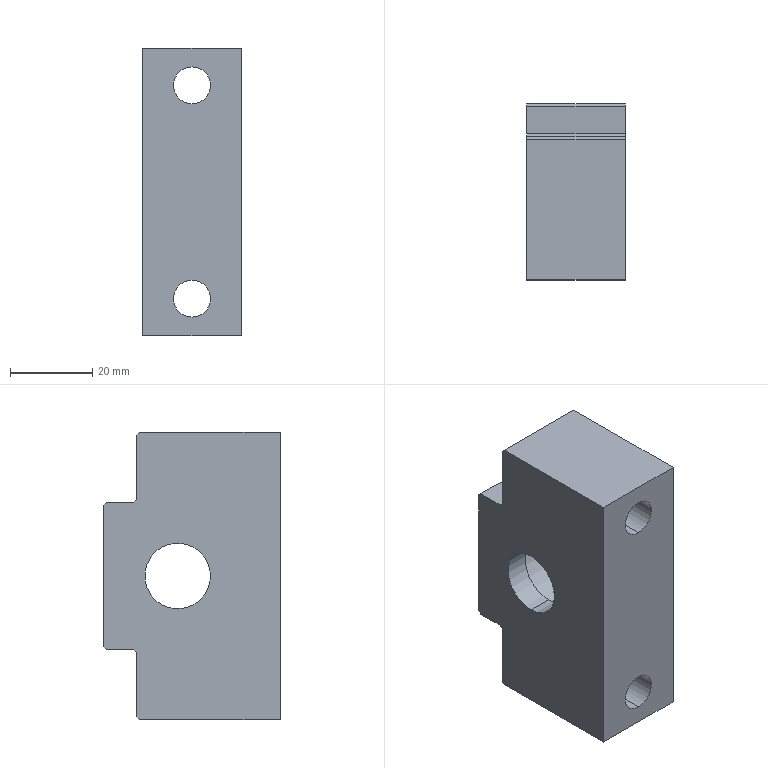Part | STEP file | BSW12bsw | 1 solid | 31 faces | box 24 x 43 x 70 mm | volume 48051 mm3 | plane 19 | cylinder 12 | commonest cylinder face diameters 9 x4 14 x4 16 x2 26.6 x2
STEP:
#1=CARTESIAN_POINT('',(12.,-25.,21.5));
#2=VERTEX_POINT('',#1);
#3=CARTESIAN_POINT('',(12.,-25.,30.5));
#4=VERTEX_POINT('',#3);
#5=CARTESIAN_POINT('',(12.,-25.,26.));
#6=DIRECTION('',(0.,1.,0.));
#7=DIRECTION('',(0.,0.,1.));
#8=AXIS2_PLACEMENT_3D('',#5,#6,#7);
#9=CIRCLE('',#8,4.5);
#10=EDGE_CURVE('',#2,#4,#9,.T.);
#11=ORIENTED_EDGE('',*,*,#10,.F.);
#12=CARTESIAN_POINT('',(12.,-1.,21.5));
#13=VERTEX_POINT('',#12);
#14=CARTESIAN_POINT('',(12.,-25.,21.5));
#15=DIRECTION('',(0.,1.,0.));
#16=VECTOR('',#15,1000.);
#17=LINE('',#14,#16);
#18=EDGE_CURVE('',#2,#13,#17,.T.);
#19=ORIENTED_EDGE('',*,*,#18,.T.);
#20=CARTESIAN_POINT('',(12.,-1.,30.5));
#21=VERTEX_POINT('',#20);
#22=CARTESIAN_POINT('',(12.,-1.,26.));
#23=DIRECTION('',(0.,1.,0.));
#24=DIRECTION('',(0.,0.,1.));
#25=AXIS2_PLACEMENT_3D('',#22,#23,#24);
#26=CIRCLE('',#25,4.5);
#27=EDGE_CURVE('',#13,#21,#26,.T.);
#28=ORIENTED_EDGE('',*,*,#27,.T.);
#29=CARTESIAN_POINT('',(12.,-25.,30.5));
#30=DIRECTION('',(0.,1.,0.));
#31=VECTOR('',#30,1000.);
#32=LINE('',#29,#31);
#33=EDGE_CURVE('',#4,#21,#32,.T.);
#34=ORIENTED_EDGE('',*,*,#33,.F.);
#35=EDGE_LOOP('',(#11,#19,#28,#34));
#36=FACE_OUTER_BOUND('',#35,.T.);
#37=CARTESIAN_POINT('',(12.,-25.,26.));
#38=DIRECTION('',(0.,1.,0.));
#39=DIRECTION('',(0.,0.,1.));
#40=AXIS2_PLACEMENT_3D('',#37,#38,#39);
#41=CYLINDRICAL_SURFACE('',#40,4.5);
#42=ADVANCED_FACE('',(#36),#41,.F.);
#43=CARTESIAN_POINT('',(12.,-1.,19.));
#44=VERTEX_POINT('',#43);
#45=CARTESIAN_POINT('',(12.,-1.,33.));
#46=VERTEX_POINT('',#45);
#47=CARTESIAN_POINT('',(12.,-1.,26.));
#48=DIRECTION('',(0.,1.,0.));
#49=DIRECTION('',(0.,0.,1.));
#50=AXIS2_PLACEMENT_3D('',#47,#48,#49);
#51=CIRCLE('',#50,7.);
#52=EDGE_CURVE('',#44,#46,#51,.T.);
#53=ORIENTED_EDGE('',*,*,#52,.F.);
#54=CARTESIAN_POINT('',(12.,10.,19.));
#55=VERTEX_POINT('',#54);
#56=CARTESIAN_POINT('',(12.,-25.,19.));
#57=DIRECTION('',(0.,1.,0.));
#58=VECTOR('',#57,1000.);
#59=LINE('',#56,#58);
#60=EDGE_CURVE('',#44,#55,#59,.T.);
#61=ORIENTED_EDGE('',*,*,#60,.T.);
#62=CARTESIAN_POINT('',(12.,10.,33.));
#63=VERTEX_POINT('',#62);
#64=CARTESIAN_POINT('',(12.,10.,26.));
#65=DIRECTION('',(0.,1.,0.));
#66=DIRECTION('',(0.,0.,1.));
#67=AXIS2_PLACEMENT_3D('',#64,#65,#66);
#68=CIRCLE('',#67,7.);
#69=EDGE_CURVE('',#55,#63,#68,.T.);
#70=ORIENTED_EDGE('',*,*,#69,.T.);
#71=CARTESIAN_POINT('',(12.,-25.,33.));
#72=DIRECTION('',(0.,1.,0.));
#73=VECTOR('',#72,1000.);
#74=LINE('',#71,#73);
#75=EDGE_CURVE('',#46,#63,#74,.T.);
#76=ORIENTED_EDGE('',*,*,#75,.F.);
#77=EDGE_LOOP('',(#53,#61,#70,#76));
#78=FACE_OUTER_BOUND('',#77,.T.);
#79=CARTESIAN_POINT('',(12.,-25.,26.));
#80=DIRECTION('',(0.,1.,0.));
#81=DIRECTION('',(0.,0.,1.));
#82=AXIS2_PLACEMENT_3D('',#79,#80,#81);
#83=CYLINDRICAL_SURFACE('',#82,7.);
#84=ADVANCED_FACE('',(#78),#83,.F.);
#85=CARTESIAN_POINT('',(12.,-25.,-30.5));
#86=VERTEX_POINT('',#85);
#87=CARTESIAN_POINT('',(12.,-25.,-21.5));
#88=VERTEX_POINT('',#87);
#89=CARTESIAN_POINT('',(12.,-25.,-26.));
#90=DIRECTION('',(0.,1.,0.));
#91=DIRECTION('',(0.,0.,1.));
#92=AXIS2_PLACEMENT_3D('',#89,#90,#91);
#93=CIRCLE('',#92,4.5);
#94=EDGE_CURVE('',#86,#88,#93,.T.);
#95=ORIENTED_EDGE('',*,*,#94,.F.);
#96=CARTESIAN_POINT('',(12.,-1.,-30.5));
#97=VERTEX_POINT('',#96);
#98=CARTESIAN_POINT('',(12.,-25.,-30.5));
#99=DIRECTION('',(0.,1.,0.));
#100=VECTOR('',#99,1000.);
#101=LINE('',#98,#100);
#102=EDGE_CURVE('',#86,#97,#101,.T.);
#103=ORIENTED_EDGE('',*,*,#102,.T.);
#104=CARTESIAN_POINT('',(12.,-1.,-21.5));
#105=VERTEX_POINT('',#104);
#106=CARTESIAN_POINT('',(12.,-1.,-26.));
#107=DIRECTION('',(0.,1.,0.));
#108=DIRECTION('',(0.,0.,1.));
#109=AXIS2_PLACEMENT_3D('',#106,#107,#108);
#110=CIRCLE('',#109,4.5);
#111=EDGE_CURVE('',#97,#105,#110,.T.);
#112=ORIENTED_EDGE('',*,*,#111,.T.);
#113=CARTESIAN_POINT('',(12.,-25.,-21.5));
#114=DIRECTION('',(0.,1.,0.));
#115=VECTOR('',#114,1000.);
#116=LINE('',#113,#115);
#117=EDGE_CURVE('',#88,#105,#116,.T.);
#118=ORIENTED_EDGE('',*,*,#117,.F.);
#119=EDGE_LOOP('',(#95,#103,#112,#118));
#120=FACE_OUTER_BOUND('',#119,.T.);
#121=CARTESIAN_POINT('',(12.,-25.,-26.));
#122=DIRECTION('',(0.,1.,0.));
#123=DIRECTION('',(0.,0.,1.));
#124=AXIS2_PLACEMENT_3D('',#121,#122,#123);
#125=CYLINDRICAL_SURFACE('',#124,4.5);
#126=ADVANCED_FACE('',(#120),#125,.F.);
#127=CARTESIAN_POINT('',(12.,-1.,-33.));
#128=VERTEX_POINT('',#127);
#129=CARTESIAN_POINT('',(12.,-1.,-19.));
#130=VERTEX_POINT('',#129);
#131=CARTESIAN_POINT('',(12.,-1.,-26.));
#132=DIRECTION('',(0.,1.,0.));
#133=DIRECTION('',(0.,0.,1.));
#134=AXIS2_PLACEMENT_3D('',#131,#132,#133);
#135=CIRCLE('',#134,7.);
#136=EDGE_CURVE('',#128,#130,#135,.T.);
#137=ORIENTED_EDGE('',*,*,#136,.F.);
#138=CARTESIAN_POINT('',(12.,10.,-33.));
#139=VERTEX_POINT('',#138);
#140=CARTESIAN_POINT('',(12.,-25.,-33.));
#141=DIRECTION('',(0.,1.,0.));
#142=VECTOR('',#141,1000.);
#143=LINE('',#140,#142);
#144=EDGE_CURVE('',#128,#139,#143,.T.);
#145=ORIENTED_EDGE('',*,*,#144,.T.);
#146=CARTESIAN_POINT('',(12.,10.,-19.));
#147=VERTEX_POINT('',#146);
#148=CARTESIAN_POINT('',(12.,10.,-26.));
#149=DIRECTION('',(0.,1.,0.));
#150=DIRECTION('',(0.,0.,1.));
#151=AXIS2_PLACEMENT_3D('',#148,#149,#150);
#152=CIRCLE('',#151,7.);
#153=EDGE_CURVE('',#139,#147,#152,.T.);
#154=ORIENTED_EDGE('',*,*,#153,.T.);
#155=CARTESIAN_POINT('',(12.,-25.,-19.));
#156=DIRECTION('',(0.,1.,0.));
#157=VECTOR('',#156,1000.);
#158=LINE('',#155,#157);
#159=EDGE_CURVE('',#130,#147,#158,.T.);
#160=ORIENTED_EDGE('',*,*,#159,.F.);
#161=EDGE_LOOP('',(#137,#145,#154,#160));
#162=FACE_OUTER_BOUND('',#161,.T.);
#163=CARTESIAN_POINT('',(12.,-25.,-26.));
#164=DIRECTION('',(0.,1.,0.));
#165=DIRECTION('',(0.,0.,1.));
#166=AXIS2_PLACEMENT_3D('',#163,#164,#165);
#167=CYLINDRICAL_SURFACE('',#166,7.);
#168=ADVANCED_FACE('',(#162),#167,.F.);
#169=CARTESIAN_POINT('',(24.,0.,-13.3));
#170=VERTEX_POINT('',#169);
#171=CARTESIAN_POINT('',(24.,0.,13.3));
#172=VERTEX_POINT('',#171);
#173=CARTESIAN_POINT('',(24.,0.,0.));
#174=DIRECTION('',(-1.,0.,0.));
#175=DIRECTION('',(0.,0.,1.));
#176=AXIS2_PLACEMENT_3D('',#173,#174,#175);
#177=CIRCLE('',#176,13.3);
#178=EDGE_CURVE('',#170,#172,#177,.T.);
#179=ORIENTED_EDGE('',*,*,#178,.F.);
#180=CARTESIAN_POINT('',(6.,0.,-13.3));
#181=VERTEX_POINT('',#180);
#182=CARTESIAN_POINT('',(24.,0.,-13.3));
#183=DIRECTION('',(-1.,0.,0.));
#184=VECTOR('',#183,1000.);
#185=LINE('',#182,#184);
#186=EDGE_CURVE('',#170,#181,#185,.T.);
#187=ORIENTED_EDGE('',*,*,#186,.T.);
#188=CARTESIAN_POINT('',(6.,0.,13.3));
#189=VERTEX_POINT('',#188);
#190=CARTESIAN_POINT('',(6.,0.,0.));
#191=DIRECTION('',(-1.,0.,0.));
#192=DIRECTION('',(0.,0.,1.));
#193=AXIS2_PLACEMENT_3D('',#190,#191,#192);
#194=CIRCLE('',#193,13.3);
#195=EDGE_CURVE('',#181,#189,#194,.T.);
#196=ORIENTED_EDGE('',*,*,#195,.T.);
#197=CARTESIAN_POINT('',(24.,0.,13.3));
#198=DIRECTION('',(-1.,0.,0.));
#199=VECTOR('',#198,1000.);
#200=LINE('',#197,#199);
#201=EDGE_CURVE('',#172,#189,#200,.T.);
#202=ORIENTED_EDGE('',*,*,#201,.F.);
#203=EDGE_LOOP('',(#179,#187,#196,#202));
#204=FACE_OUTER_BOUND('',#203,.T.);
#205=CARTESIAN_POINT('',(24.,0.,0.));
#206=DIRECTION('',(-1.,0.,0.));
#207=DIRECTION('',(0.,0.,1.));
#208=AXIS2_PLACEMENT_3D('',#205,#206,#207);
#209=CYLINDRICAL_SURFACE('',#208,13.3);
#210=ADVANCED_FACE('',(#204),#209,.F.);
#211=CARTESIAN_POINT('',(6.,0.,-8.));
#212=VERTEX_POINT('',#211);
#213=CARTESIAN_POINT('',(6.,0.,8.));
#214=VERTEX_POINT('',#213);
#215=CARTESIAN_POINT('',(6.,0.,0.));
#216=DIRECTION('',(-1.,0.,0.));
#217=DIRECTION('',(0.,0.,1.));
#218=AXIS2_PLACEMENT_3D('',#215,#216,#217);
#219=CIRCLE('',#218,8.);
#220=EDGE_CURVE('',#212,#214,#219,.T.);
#221=ORIENTED_EDGE('',*,*,#220,.F.);
#222=CARTESIAN_POINT('',(0.,0.,-8.));
#223=VERTEX_POINT('',#222);
#224=CARTESIAN_POINT('',(24.,0.,-8.));
#225=DIRECTION('',(-1.,0.,0.));
#226=VECTOR('',#225,1000.);
#227=LINE('',#224,#226);
#228=EDGE_CURVE('',#212,#223,#227,.T.);
#229=ORIENTED_EDGE('',*,*,#228,.T.);
#230=CARTESIAN_POINT('',(0.,0.,8.));
#231=VERTEX_POINT('',#230);
#232=CARTESIAN_POINT('',(0.,0.,0.));
#233=DIRECTION('',(-1.,0.,0.));
#234=DIRECTION('',(0.,0.,1.));
#235=AXIS2_PLACEMENT_3D('',#232,#233,#234);
#236=CIRCLE('',#235,8.);
#237=EDGE_CURVE('',#223,#231,#236,.T.);
#238=ORIENTED_EDGE('',*,*,#237,.T.);
#239=CARTESIAN_POINT('',(24.,0.,8.));
#240=DIRECTION('',(-1.,0.,0.));
#241=VECTOR('',#240,1000.);
#242=LINE('',#239,#241);
#243=EDGE_CURVE('',#214,#231,#242,.T.);
#244=ORIENTED_EDGE('',*,*,#243,.F.);
#245=EDGE_LOOP('',(#221,#229,#238,#244));
#246=FACE_OUTER_BOUND('',#245,.T.);
#247=CARTESIAN_POINT('',(24.,0.,0.));
#248=DIRECTION('',(-1.,0.,0.));
#249=DIRECTION('',(0.,0.,1.));
#250=AXIS2_PLACEMENT_3D('',#247,#248,#249);
#251=CYLINDRICAL_SURFACE('',#250,8.);
#252=ADVANCED_FACE('',(#246),#251,.F.);
#253=CARTESIAN_POINT('',(12.,-25.,-26.));
#254=DIRECTION('',(0.,1.,0.));
#255=DIRECTION('',(0.,0.,1.));
#256=AXIS2_PLACEMENT_3D('',#253,#254,#255);
#257=CIRCLE('',#256,4.5);
#258=EDGE_CURVE('',#88,#86,#257,.T.);
#259=ORIENTED_EDGE('',*,*,#258,.T.);
#260=ORIENTED_EDGE('',*,*,#94,.T.);
#261=EDGE_LOOP('',(#259,#260));
#262=FACE_BOUND('',#261,.T.);
#263=CARTESIAN_POINT('',(0.,-25.,35.));
#264=VERTEX_POINT('',#263);
#265=CARTESIAN_POINT('',(0.,-25.,-35.));
#266=VERTEX_POINT('',#265);
#267=CARTESIAN_POINT('',(0.,-25.,35.));
#268=DIRECTION('',(0.,0.,-1.));
#269=VECTOR('',#268,1000.);
#270=LINE('',#267,#269);
#271=EDGE_CURVE('',#264,#266,#270,.T.);
#272=ORIENTED_EDGE('',*,*,#271,.T.);
#273=CARTESIAN_POINT('',(24.,-25.,-35.));
#274=VERTEX_POINT('',#273);
#275=CARTESIAN_POINT('',(24.,-25.,-35.));
#276=DIRECTION('',(-1.,0.,0.));
#277=VECTOR('',#276,1000.);
#278=LINE('',#275,#277);
#279=EDGE_CURVE('',#274,#266,#278,.T.);
#280=ORIENTED_EDGE('',*,*,#279,.F.);
#281=CARTESIAN_POINT('',(24.,-25.,35.));
#282=VERTEX_POINT('',#281);
#283=CARTESIAN_POINT('',(24.,-25.,35.));
#284=DIRECTION('',(0.,0.,-1.));
#285=VECTOR('',#284,1000.);
#286=LINE('',#283,#285);
#287=EDGE_CURVE('',#282,#274,#286,.T.);
#288=ORIENTED_EDGE('',*,*,#287,.F.);
#289=CARTESIAN_POINT('',(24.,-25.,35.));
#290=DIRECTION('',(-1.,0.,0.));
#291=VECTOR('',#290,1000.);
#292=LINE('',#289,#291);
#293=EDGE_CURVE('',#282,#264,#292,.T.);
#294=ORIENTED_EDGE('',*,*,#293,.T.);
#295=EDGE_LOOP('',(#272,#280,#288,#294));
#296=FACE_OUTER_BOUND('',#295,.T.);
#297=CARTESIAN_POINT('',(12.,-25.,26.));
#298=DIRECTION('',(0.,1.,0.));
#299=DIRECTION('',(0.,0.,1.));
#300=AXIS2_PLACEMENT_3D('',#297,#298,#299);
#301=CIRCLE('',#300,4.5);
#302=EDGE_CURVE('',#4,#2,#301,.T.);
#303=ORIENTED_EDGE('',*,*,#302,.T.);
#304=ORIENTED_EDGE('',*,*,#10,.T.);
#305=EDGE_LOOP('',(#303,#304));
#306=FACE_BOUND('',#305,.T.);
#307=CARTESIAN_POINT('',(24.,-25.,35.));
#308=DIRECTION('',(0.,1.,0.));
#309=DIRECTION('',(0.,0.,1.));
#310=AXIS2_PLACEMENT_3D('',#307,#308,#309);
#311=PLANE('',#310);
#312=ADVANCED_FACE('',(#262,#296,#306),#311,.F.);
#313=CARTESIAN_POINT('',(0.,10.,18.7));
#314=VERTEX_POINT('',#313);
#315=CARTESIAN_POINT('',(0.,10.,34.3));
#316=VERTEX_POINT('',#315);
#317=CARTESIAN_POINT('',(0.,10.,18.7));
#318=DIRECTION('',(0.,0.,1.));
#319=VECTOR('',#318,1000.);
#320=LINE('',#317,#319);
#321=EDGE_CURVE('',#314,#316,#320,.T.);
#322=ORIENTED_EDGE('',*,*,#321,.T.);
#323=CARTESIAN_POINT('',(24.,10.,34.3));
#324=VERTEX_POINT('',#323);
#325=CARTESIAN_POINT('',(24.,10.,34.3));
#326=DIRECTION('',(-1.,0.,0.));
#327=VECTOR('',#326,1000.);
#328=LINE('',#325,#327);
#329=EDGE_CURVE('',#324,#316,#328,.T.);
#330=ORIENTED_EDGE('',*,*,#329,.F.);
#331=CARTESIAN_POINT('',(24.,10.,18.7));
#332=VERTEX_POINT('',#331);
#333=CARTESIAN_POINT('',(24.,10.,18.7));
#334=DIRECTION('',(0.,0.,1.));
#335=VECTOR('',#334,1000.);
#336=LINE('',#333,#335);
#337=EDGE_CURVE('',#332,#324,#336,.T.);
#338=ORIENTED_EDGE('',*,*,#337,.F.);
#339=CARTESIAN_POINT('',(24.,10.,18.7));
#340=DIRECTION('',(-1.,0.,0.));
#341=VECTOR('',#340,1000.);
#342=LINE('',#339,#341);
#343=EDGE_CURVE('',#332,#314,#342,.T.);
#344=ORIENTED_EDGE('',*,*,#343,.T.);
#345=EDGE_LOOP('',(#322,#330,#338,#344));
#346=FACE_OUTER_BOUND('',#345,.T.);
#347=CARTESIAN_POINT('',(12.,10.,26.));
#348=DIRECTION('',(0.,1.,0.));
#349=DIRECTION('',(0.,0.,1.));
#350=AXIS2_PLACEMENT_3D('',#347,#348,#349);
#351=CIRCLE('',#350,7.);
#352=EDGE_CURVE('',#63,#55,#351,.T.);
#353=ORIENTED_EDGE('',*,*,#352,.F.);
#354=ORIENTED_EDGE('',*,*,#69,.F.);
#355=EDGE_LOOP('',(#353,#354));
#356=FACE_BOUND('',#355,.T.);
#357=CARTESIAN_POINT('',(24.,10.,18.7));
#358=DIRECTION('',(0.,-1.,0.));
#359=DIRECTION('',(0.,0.,-1.));
#360=AXIS2_PLACEMENT_3D('',#357,#358,#359);
#361=PLANE('',#360);
#362=ADVANCED_FACE('',(#346,#356),#361,.F.);
#363=CARTESIAN_POINT('',(0.,10.,-34.3));
#364=VERTEX_POINT('',#363);
#365=CARTESIAN_POINT('',(0.,10.,-18.7));
#366=VERTEX_POINT('',#365);
#367=CARTESIAN_POINT('',(0.,10.,-34.3));
#368=DIRECTION('',(0.,0.,1.));
#369=VECTOR('',#368,1000.);
#370=LINE('',#367,#369);
#371=EDGE_CURVE('',#364,#366,#370,.T.);
#372=ORIENTED_EDGE('',*,*,#371,.T.);
#373=CARTESIAN_POINT('',(24.,10.,-18.7));
#374=VERTEX_POINT('',#373);
#375=CARTESIAN_POINT('',(24.,10.,-18.7));
#376=DIRECTION('',(-1.,0.,0.));
#377=VECTOR('',#376,1000.);
#378=LINE('',#375,#377);
#379=EDGE_CURVE('',#374,#366,#378,.T.);
#380=ORIENTED_EDGE('',*,*,#379,.F.);
#381=CARTESIAN_POINT('',(24.,10.,-34.3));
#382=VERTEX_POINT('',#381);
#383=CARTESIAN_POINT('',(24.,10.,-34.3));
#384=DIRECTION('',(0.,0.,1.));
#385=VECTOR('',#384,1000.);
#386=LINE('',#383,#385);
#387=EDGE_CURVE('',#382,#374,#386,.T.);
#388=ORIENTED_EDGE('',*,*,#387,.F.);
#389=CARTESIAN_POINT('',(24.,10.,-34.3));
#390=DIRECTION('',(-1.,0.,0.));
#391=VECTOR('',#390,1000.);
#392=LINE('',#389,#391);
#393=EDGE_CURVE('',#382,#364,#392,.T.);
#394=ORIENTED_EDGE('',*,*,#393,.T.);
#395=EDGE_LOOP('',(#372,#380,#388,#394));
#396=FACE_OUTER_BOUND('',#395,.T.);
#397=CARTESIAN_POINT('',(12.,10.,-26.));
#398=DIRECTION('',(0.,1.,0.));
#399=DIRECTION('',(0.,0.,1.));
#400=AXIS2_PLACEMENT_3D('',#397,#398,#399);
#401=CIRCLE('',#400,7.);
#402=EDGE_CURVE('',#147,#139,#401,.T.);
#403=ORIENTED_EDGE('',*,*,#402,.F.);
#404=ORIENTED_EDGE('',*,*,#153,.F.);
#405=EDGE_LOOP('',(#403,#404));
#406=FACE_BOUND('',#405,.T.);
#407=CARTESIAN_POINT('',(24.,10.,-34.3));
#408=DIRECTION('',(0.,-1.,0.));
#409=DIRECTION('',(0.,0.,-1.));
#410=AXIS2_PLACEMENT_3D('',#407,#408,#409);
#411=PLANE('',#410);
#412=ADVANCED_FACE('',(#396,#406),#411,.F.);
#413=CARTESIAN_POINT('',(24.,9.3,35.));
#414=VERTEX_POINT('',#413);
#415=CARTESIAN_POINT('',(24.,9.3,35.));
#416=DIRECTION('',(0.,-1.,0.));
#417=VECTOR('',#416,1000.);
#418=LINE('',#415,#417);
#419=EDGE_CURVE('',#414,#282,#418,.T.);
#420=ORIENTED_EDGE('',*,*,#419,.T.);
#421=ORIENTED_EDGE('',*,*,#287,.T.);
#422=CARTESIAN_POINT('',(24.,9.3,-35.));
#423=VERTEX_POINT('',#422);
#424=CARTESIAN_POINT('',(24.,-25.,-35.));
#425=DIRECTION('',(0.,1.,0.));
#426=VECTOR('',#425,1000.);
#427=LINE('',#424,#426);
#428=EDGE_CURVE('',#274,#423,#427,.T.);
#429=ORIENTED_EDGE('',*,*,#428,.T.);
#430=CARTESIAN_POINT('',(24.,9.3,-35.));
#431=DIRECTION('',(0.,0.7071,0.7071));
#432=VECTOR('',#431,1000.);
#433=LINE('',#430,#432);
#434=EDGE_CURVE('',#423,#382,#433,.T.);
#435=ORIENTED_EDGE('',*,*,#434,.T.);
#436=ORIENTED_EDGE('',*,*,#387,.T.);
#437=CARTESIAN_POINT('',(24.,10.7,-18.));
#438=VERTEX_POINT('',#437);
#439=CARTESIAN_POINT('',(24.,10.,-18.7));
#440=DIRECTION('',(0.,0.7071,0.7071));
#441=VECTOR('',#440,1000.);
#442=LINE('',#439,#441);
#443=EDGE_CURVE('',#374,#438,#442,.T.);
#444=ORIENTED_EDGE('',*,*,#443,.T.);
#445=CARTESIAN_POINT('',(24.,17.3,-18.));
#446=VERTEX_POINT('',#445);
#447=CARTESIAN_POINT('',(24.,10.7,-18.));
#448=DIRECTION('',(0.,1.,0.));
#449=VECTOR('',#448,1000.);
#450=LINE('',#447,#449);
#451=EDGE_CURVE('',#438,#446,#450,.T.);
#452=ORIENTED_EDGE('',*,*,#451,.T.);
#453=CARTESIAN_POINT('',(24.,18.,-17.3));
#454=VERTEX_POINT('',#453);
#455=CARTESIAN_POINT('',(24.,17.3,-18.));
#456=DIRECTION('',(0.,0.7071,0.7071));
#457=VECTOR('',#456,1000.);
#458=LINE('',#455,#457);
#459=EDGE_CURVE('',#446,#454,#458,.T.);
#460=ORIENTED_EDGE('',*,*,#459,.T.);
#461=CARTESIAN_POINT('',(24.,18.,17.3));
#462=VERTEX_POINT('',#461);
#463=CARTESIAN_POINT('',(24.,18.,-17.3));
#464=DIRECTION('',(0.,0.,1.));
#465=VECTOR('',#464,1000.);
#466=LINE('',#463,#465);
#467=EDGE_CURVE('',#454,#462,#466,.T.);
#468=ORIENTED_EDGE('',*,*,#467,.T.);
#469=CARTESIAN_POINT('',(24.,17.3,18.));
#470=VERTEX_POINT('',#469);
#471=CARTESIAN_POINT('',(24.,18.,17.3));
#472=DIRECTION('',(0.,-0.7071,0.7071));
#473=VECTOR('',#472,1000.);
#474=LINE('',#471,#473);
#475=EDGE_CURVE('',#462,#470,#474,.T.);
#476=ORIENTED_EDGE('',*,*,#475,.T.);
#477=CARTESIAN_POINT('',(24.,10.7,18.));
#478=VERTEX_POINT('',#477);
#479=CARTESIAN_POINT('',(24.,17.3,18.));
#480=DIRECTION('',(0.,-1.,0.));
#481=VECTOR('',#480,1000.);
#482=LINE('',#479,#481);
#483=EDGE_CURVE('',#470,#478,#482,.T.);
#484=ORIENTED_EDGE('',*,*,#483,.T.);
#485=CARTESIAN_POINT('',(24.,10.7,18.));
#486=DIRECTION('',(0.,-0.7071,0.7071));
#487=VECTOR('',#486,1000.);
#488=LINE('',#485,#487);
#489=EDGE_CURVE('',#478,#332,#488,.T.);
#490=ORIENTED_EDGE('',*,*,#489,.T.);
#491=ORIENTED_EDGE('',*,*,#337,.T.);
#492=CARTESIAN_POINT('',(24.,10.,34.3));
#493=DIRECTION('',(0.,-0.7071,0.7071));
#494=VECTOR('',#493,1000.);
#495=LINE('',#492,#494);
#496=EDGE_CURVE('',#324,#414,#495,.T.);
#497=ORIENTED_EDGE('',*,*,#496,.T.);
#498=EDGE_LOOP('',(#420,#421,#429,#435,#436,#444,#452,#460,#468,#476,#484,#490,#491,#497));
#499=FACE_OUTER_BOUND('',#498,.T.);
#500=CARTESIAN_POINT('',(24.,0.,0.));
#501=DIRECTION('',(-1.,0.,0.));
#502=DIRECTION('',(0.,0.,1.));
#503=AXIS2_PLACEMENT_3D('',#500,#501,#502);
#504=CIRCLE('',#503,13.3);
#505=EDGE_CURVE('',#172,#170,#504,.T.);
#506=ORIENTED_EDGE('',*,*,#505,.T.);
#507=ORIENTED_EDGE('',*,*,#178,.T.);
#508=EDGE_LOOP('',(#506,#507));
#509=FACE_BOUND('',#508,.T.);
#510=CARTESIAN_POINT('',(24.,-25.,35.));
#511=DIRECTION('',(1.,0.,0.));
#512=DIRECTION('',(0.,0.,-1.));
#513=AXIS2_PLACEMENT_3D('',#510,#511,#512);
#514=PLANE('',#513);
#515=ADVANCED_FACE('',(#499,#509),#514,.T.);
#516=CARTESIAN_POINT('',(0.,9.3,35.));
#517=VERTEX_POINT('',#516);
#518=CARTESIAN_POINT('',(0.,9.3,35.));
#519=DIRECTION('',(0.,-1.,0.));
#520=VECTOR('',#519,1000.);
#521=LINE('',#518,#520);
#522=EDGE_CURVE('',#517,#264,#521,.T.);
#523=ORIENTED_EDGE('',*,*,#522,.F.);
#524=CARTESIAN_POINT('',(0.,10.,34.3));
#525=DIRECTION('',(0.,-0.7071,0.7071));
#526=VECTOR('',#525,1000.);
#527=LINE('',#524,#526);
#528=EDGE_CURVE('',#316,#517,#527,.T.);
#529=ORIENTED_EDGE('',*,*,#528,.F.);
#530=ORIENTED_EDGE('',*,*,#321,.F.);
#531=CARTESIAN_POINT('',(0.,10.7,18.));
#532=VERTEX_POINT('',#531);
#533=CARTESIAN_POINT('',(0.,10.7,18.));
#534=DIRECTION('',(0.,-0.7071,0.7071));
#535=VECTOR('',#534,1000.);
#536=LINE('',#533,#535);
#537=EDGE_CURVE('',#532,#314,#536,.T.);
#538=ORIENTED_EDGE('',*,*,#537,.F.);
#539=CARTESIAN_POINT('',(0.,17.3,18.));
#540=VERTEX_POINT('',#539);
#541=CARTESIAN_POINT('',(0.,17.3,18.));
#542=DIRECTION('',(0.,-1.,0.));
#543=VECTOR('',#542,1000.);
#544=LINE('',#541,#543);
#545=EDGE_CURVE('',#540,#532,#544,.T.);
#546=ORIENTED_EDGE('',*,*,#545,.F.);
#547=CARTESIAN_POINT('',(0.,18.,17.3));
#548=VERTEX_POINT('',#547);
#549=CARTESIAN_POINT('',(0.,18.,17.3));
#550=DIRECTION('',(0.,-0.7071,0.7071));
#551=VECTOR('',#550,1000.);
#552=LINE('',#549,#551);
#553=EDGE_CURVE('',#548,#540,#552,.T.);
#554=ORIENTED_EDGE('',*,*,#553,.F.);
#555=CARTESIAN_POINT('',(0.,18.,-17.3));
#556=VERTEX_POINT('',#555);
#557=CARTESIAN_POINT('',(0.,18.,-17.3));
#558=DIRECTION('',(0.,0.,1.));
#559=VECTOR('',#558,1000.);
#560=LINE('',#557,#559);
#561=EDGE_CURVE('',#556,#548,#560,.T.);
#562=ORIENTED_EDGE('',*,*,#561,.F.);
#563=CARTESIAN_POINT('',(0.,17.3,-18.));
#564=VERTEX_POINT('',#563);
#565=CARTESIAN_POINT('',(0.,17.3,-18.));
#566=DIRECTION('',(0.,0.7071,0.7071));
#567=VECTOR('',#566,1000.);
#568=LINE('',#565,#567);
#569=EDGE_CURVE('',#564,#556,#568,.T.);
#570=ORIENTED_EDGE('',*,*,#569,.F.);
#571=CARTESIAN_POINT('',(0.,10.7,-18.));
#572=VERTEX_POINT('',#571);
#573=CARTESIAN_POINT('',(0.,10.7,-18.));
#574=DIRECTION('',(0.,1.,0.));
#575=VECTOR('',#574,1000.);
#576=LINE('',#573,#575);
#577=EDGE_CURVE('',#572,#564,#576,.T.);
#578=ORIENTED_EDGE('',*,*,#577,.F.);
#579=CARTESIAN_POINT('',(0.,10.,-18.7));
#580=DIRECTION('',(0.,0.7071,0.7071));
#581=VECTOR('',#580,1000.);
#582=LINE('',#579,#581);
#583=EDGE_CURVE('',#366,#572,#582,.T.);
#584=ORIENTED_EDGE('',*,*,#583,.F.);
#585=ORIENTED_EDGE('',*,*,#371,.F.);
#586=CARTESIAN_POINT('',(0.,9.3,-35.));
#587=VERTEX_POINT('',#586);
#588=CARTESIAN_POINT('',(0.,9.3,-35.));
#589=DIRECTION('',(0.,0.7071,0.7071));
#590=VECTOR('',#589,1000.);
#591=LINE('',#588,#590);
#592=EDGE_CURVE('',#587,#364,#591,.T.);
#593=ORIENTED_EDGE('',*,*,#592,.F.);
#594=CARTESIAN_POINT('',(0.,-25.,-35.));
#595=DIRECTION('',(0.,1.,0.));
#596=VECTOR('',#595,1000.);
#597=LINE('',#594,#596);
#598=EDGE_CURVE('',#266,#587,#597,.T.);
#599=ORIENTED_EDGE('',*,*,#598,.F.);
#600=ORIENTED_EDGE('',*,*,#271,.F.);
#601=EDGE_LOOP('',(#523,#529,#530,#538,#546,#554,#562,#570,#578,#584,#585,#593,#599,#600));
#602=FACE_OUTER_BOUND('',#601,.T.);
#603=CARTESIAN_POINT('',(0.,0.,0.));
#604=DIRECTION('',(-1.,0.,0.));
#605=DIRECTION('',(0.,0.,1.));
#606=AXIS2_PLACEMENT_3D('',#603,#604,#605);
#607=CIRCLE('',#606,8.);
#608=EDGE_CURVE('',#231,#223,#607,.T.);
#609=ORIENTED_EDGE('',*,*,#608,.F.);
#610=ORIENTED_EDGE('',*,*,#237,.F.);
#611=EDGE_LOOP('',(#609,#610));
#612=FACE_BOUND('',#611,.T.);
#613=CARTESIAN_POINT('',(0.,-25.,35.));
#614=DIRECTION('',(1.,0.,0.));
#615=DIRECTION('',(0.,0.,-1.));
#616=AXIS2_PLACEMENT_3D('',#613,#614,#615);
#617=PLANE('',#616);
#618=ADVANCED_FACE('',(#602,#612),#617,.F.);
#619=ORIENTED_EDGE('',*,*,#522,.T.);
#620=ORIENTED_EDGE('',*,*,#293,.F.);
#621=ORIENTED_EDGE('',*,*,#419,.F.);
#622=CARTESIAN_POINT('',(24.,9.3,35.));
#623=DIRECTION('',(-1.,0.,0.));
#624=VECTOR('',#623,1000.);
#625=LINE('',#622,#624);
#626=EDGE_CURVE('',#414,#517,#625,.T.);
#627=ORIENTED_EDGE('',*,*,#626,.T.);
#628=EDGE_LOOP('',(#619,#620,#621,#627));
#629=FACE_OUTER_BOUND('',#628,.T.);
#630=CARTESIAN_POINT('',(24.,9.3,35.));
#631=DIRECTION('',(0.,0.,-1.));
#632=DIRECTION('',(-1.,0.,0.));
#633=AXIS2_PLACEMENT_3D('',#630,#631,#632);
#634=PLANE('',#633);
#635=ADVANCED_FACE('',(#629),#634,.F.);
#636=ORIENTED_EDGE('',*,*,#598,.T.);
#637=CARTESIAN_POINT('',(24.,9.3,-35.));
#638=DIRECTION('',(-1.,0.,0.));
#639=VECTOR('',#638,1000.);
#640=LINE('',#637,#639);
#641=EDGE_CURVE('',#423,#587,#640,.T.);
#642=ORIENTED_EDGE('',*,*,#641,.F.);
#643=ORIENTED_EDGE('',*,*,#428,.F.);
#644=ORIENTED_EDGE('',*,*,#279,.T.);
#645=EDGE_LOOP('',(#636,#642,#643,#644));
#646=FACE_OUTER_BOUND('',#645,.T.);
#647=CARTESIAN_POINT('',(24.,-25.,-35.));
#648=DIRECTION('',(0.,0.,1.));
#649=DIRECTION('',(1.,0.,0.));
#650=AXIS2_PLACEMENT_3D('',#647,#648,#649);
#651=PLANE('',#650);
#652=ADVANCED_FACE('',(#646),#651,.F.);
#653=ORIENTED_EDGE('',*,*,#592,.T.);
#654=ORIENTED_EDGE('',*,*,#393,.F.);
#655=ORIENTED_EDGE('',*,*,#434,.F.);
#656=ORIENTED_EDGE('',*,*,#641,.T.);
#657=EDGE_LOOP('',(#653,#654,#655,#656));
#658=FACE_OUTER_BOUND('',#657,.T.);
#659=CARTESIAN_POINT('',(24.,9.3,-35.));
#660=DIRECTION('',(0.,-0.7071,0.7071));
#661=DIRECTION('',(0.,-0.7071,-0.7071));
#662=AXIS2_PLACEMENT_3D('',#659,#660,#661);
#663=PLANE('',#662);
#664=ADVANCED_FACE('',(#658),#663,.F.);
#665=ORIENTED_EDGE('',*,*,#583,.T.);
#666=CARTESIAN_POINT('',(24.,10.7,-18.));
#667=DIRECTION('',(-1.,0.,0.));
#668=VECTOR('',#667,1000.);
#669=LINE('',#666,#668);
#670=EDGE_CURVE('',#438,#572,#669,.T.);
#671=ORIENTED_EDGE('',*,*,#670,.F.);
#672=ORIENTED_EDGE('',*,*,#443,.F.);
#673=ORIENTED_EDGE('',*,*,#379,.T.);
#674=EDGE_LOOP('',(#665,#671,#672,#673));
#675=FACE_OUTER_BOUND('',#674,.T.);
#676=CARTESIAN_POINT('',(24.,10.,-18.7));
#677=DIRECTION('',(0.,-0.7071,0.7071));
#678=DIRECTION('',(0.,-0.7071,-0.7071));
#679=AXIS2_PLACEMENT_3D('',#676,#677,#678);
#680=PLANE('',#679);
#681=ADVANCED_FACE('',(#675),#680,.F.);
#682=ORIENTED_EDGE('',*,*,#577,.T.);
#683=CARTESIAN_POINT('',(24.,17.3,-18.));
#684=DIRECTION('',(-1.,0.,0.));
#685=VECTOR('',#684,1000.);
#686=LINE('',#683,#685);
#687=EDGE_CURVE('',#446,#564,#686,.T.);
#688=ORIENTED_EDGE('',*,*,#687,.F.);
#689=ORIENTED_EDGE('',*,*,#451,.F.);
#690=ORIENTED_EDGE('',*,*,#670,.T.);
#691=EDGE_LOOP('',(#682,#688,#689,#690));
#692=FACE_OUTER_BOUND('',#691,.T.);
#693=CARTESIAN_POINT('',(24.,10.7,-18.));
#694=DIRECTION('',(0.,0.,1.));
#695=DIRECTION('',(1.,0.,0.));
#696=AXIS2_PLACEMENT_3D('',#693,#694,#695);
#697=PLANE('',#696);
#698=ADVANCED_FACE('',(#692),#697,.F.);
#699=ORIENTED_EDGE('',*,*,#569,.T.);
#700=CARTESIAN_POINT('',(24.,18.,-17.3));
#701=DIRECTION('',(-1.,0.,0.));
#702=VECTOR('',#701,1000.);
#703=LINE('',#700,#702);
#704=EDGE_CURVE('',#454,#556,#703,.T.);
#705=ORIENTED_EDGE('',*,*,#704,.F.);
#706=ORIENTED_EDGE('',*,*,#459,.F.);
#707=ORIENTED_EDGE('',*,*,#687,.T.);
#708=EDGE_LOOP('',(#699,#705,#706,#707));
#709=FACE_OUTER_BOUND('',#708,.T.);
#710=CARTESIAN_POINT('',(24.,17.3,-18.));
#711=DIRECTION('',(0.,-0.7071,0.7071));
#712=DIRECTION('',(0.,-0.7071,-0.7071));
#713=AXIS2_PLACEMENT_3D('',#710,#711,#712);
#714=PLANE('',#713);
#715=ADVANCED_FACE('',(#709),#714,.F.);
#716=ORIENTED_EDGE('',*,*,#561,.T.);
#717=CARTESIAN_POINT('',(24.,18.,17.3));
#718=DIRECTION('',(-1.,0.,0.));
#719=VECTOR('',#718,1000.);
#720=LINE('',#717,#719);
#721=EDGE_CURVE('',#462,#548,#720,.T.);
#722=ORIENTED_EDGE('',*,*,#721,.F.);
#723=ORIENTED_EDGE('',*,*,#467,.F.);
#724=ORIENTED_EDGE('',*,*,#704,.T.);
#725=EDGE_LOOP('',(#716,#722,#723,#724));
#726=FACE_OUTER_BOUND('',#725,.T.);
#727=CARTESIAN_POINT('',(24.,18.,-17.3));
#728=DIRECTION('',(0.,-1.,0.));
#729=DIRECTION('',(0.,0.,-1.));
#730=AXIS2_PLACEMENT_3D('',#727,#728,#729);
#731=PLANE('',#730);
#732=ADVANCED_FACE('',(#726),#731,.F.);
#733=ORIENTED_EDGE('',*,*,#553,.T.);
#734=CARTESIAN_POINT('',(24.,17.3,18.));
#735=DIRECTION('',(-1.,0.,0.));
#736=VECTOR('',#735,1000.);
#737=LINE('',#734,#736);
#738=EDGE_CURVE('',#470,#540,#737,.T.);
#739=ORIENTED_EDGE('',*,*,#738,.F.);
#740=ORIENTED_EDGE('',*,*,#475,.F.);
#741=ORIENTED_EDGE('',*,*,#721,.T.);
#742=EDGE_LOOP('',(#733,#739,#740,#741));
#743=FACE_OUTER_BOUND('',#742,.T.);
#744=CARTESIAN_POINT('',(24.,18.,17.3));
#745=DIRECTION('',(0.,-0.7071,-0.7071));
#746=DIRECTION('',(0.,0.7071,-0.7071));
#747=AXIS2_PLACEMENT_3D('',#744,#745,#746);
#748=PLANE('',#747);
#749=ADVANCED_FACE('',(#743),#748,.F.);
#750=ORIENTED_EDGE('',*,*,#545,.T.);
#751=CARTESIAN_POINT('',(24.,10.7,18.));
#752=DIRECTION('',(-1.,0.,0.));
#753=VECTOR('',#752,1000.);
#754=LINE('',#751,#753);
#755=EDGE_CURVE('',#478,#532,#754,.T.);
#756=ORIENTED_EDGE('',*,*,#755,.F.);
#757=ORIENTED_EDGE('',*,*,#483,.F.);
#758=ORIENTED_EDGE('',*,*,#738,.T.);
#759=EDGE_LOOP('',(#750,#756,#757,#758));
#760=FACE_OUTER_BOUND('',#759,.T.);
#761=CARTESIAN_POINT('',(24.,17.3,18.));
#762=DIRECTION('',(0.,0.,-1.));
#763=DIRECTION('',(-1.,0.,0.));
#764=AXIS2_PLACEMENT_3D('',#761,#762,#763);
#765=PLANE('',#764);
#766=ADVANCED_FACE('',(#760),#765,.F.);
#767=ORIENTED_EDGE('',*,*,#537,.T.);
#768=ORIENTED_EDGE('',*,*,#343,.F.);
#769=ORIENTED_EDGE('',*,*,#489,.F.);
#770=ORIENTED_EDGE('',*,*,#755,.T.);
#771=EDGE_LOOP('',(#767,#768,#769,#770));
#772=FACE_OUTER_BOUND('',#771,.T.);
#773=CARTESIAN_POINT('',(24.,10.7,18.));
#774=DIRECTION('',(0.,-0.7071,-0.7071));
#775=DIRECTION('',(0.,0.7071,-0.7071));
#776=AXIS2_PLACEMENT_3D('',#773,#774,#775);
#777=PLANE('',#776);
#778=ADVANCED_FACE('',(#772),#777,.F.);
#779=ORIENTED_EDGE('',*,*,#528,.T.);
#780=ORIENTED_EDGE('',*,*,#626,.F.);
#781=ORIENTED_EDGE('',*,*,#496,.F.);
#782=ORIENTED_EDGE('',*,*,#329,.T.);
#783=EDGE_LOOP('',(#779,#780,#781,#782));
#784=FACE_OUTER_BOUND('',#783,.T.);
#785=CARTESIAN_POINT('',(24.,10.,34.3));
#786=DIRECTION('',(0.,-0.7071,-0.7071));
#787=DIRECTION('',(0.,0.7071,-0.7071));
#788=AXIS2_PLACEMENT_3D('',#785,#786,#787);
#789=PLANE('',#788);
#790=ADVANCED_FACE('',(#784),#789,.F.);
#791=ORIENTED_EDGE('',*,*,#228,.F.);
#792=CARTESIAN_POINT('',(6.,0.,0.));
#793=DIRECTION('',(-1.,0.,0.));
#794=DIRECTION('',(0.,0.,1.));
#795=AXIS2_PLACEMENT_3D('',#792,#793,#794);
#796=CIRCLE('',#795,8.);
#797=EDGE_CURVE('',#214,#212,#796,.T.);
#798=ORIENTED_EDGE('',*,*,#797,.F.);
#799=ORIENTED_EDGE('',*,*,#243,.T.);
#800=ORIENTED_EDGE('',*,*,#608,.T.);
#801=EDGE_LOOP('',(#791,#798,#799,#800));
#802=FACE_OUTER_BOUND('',#801,.T.);
#803=CARTESIAN_POINT('',(24.,0.,0.));
#804=DIRECTION('',(-1.,0.,0.));
#805=DIRECTION('',(0.,0.,1.));
#806=AXIS2_PLACEMENT_3D('',#803,#804,#805);
#807=CYLINDRICAL_SURFACE('',#806,8.);
#808=ADVANCED_FACE('',(#802),#807,.F.);
#809=ORIENTED_EDGE('',*,*,#797,.T.);
#810=ORIENTED_EDGE('',*,*,#220,.T.);
#811=EDGE_LOOP('',(#809,#810));
#812=FACE_BOUND('',#811,.T.);
#813=CARTESIAN_POINT('',(6.,0.,0.));
#814=DIRECTION('',(-1.,0.,0.));
#815=DIRECTION('',(0.,0.,1.));
#816=AXIS2_PLACEMENT_3D('',#813,#814,#815);
#817=CIRCLE('',#816,13.3);
#818=EDGE_CURVE('',#189,#181,#817,.T.);
#819=ORIENTED_EDGE('',*,*,#818,.F.);
#820=ORIENTED_EDGE('',*,*,#195,.F.);
#821=EDGE_LOOP('',(#819,#820));
#822=FACE_OUTER_BOUND('',#821,.T.);
#823=CARTESIAN_POINT('',(6.,8.,0.));
#824=DIRECTION('',(1.,0.,0.));
#825=DIRECTION('',(0.,0.,-1.));
#826=AXIS2_PLACEMENT_3D('',#823,#824,#825);
#827=PLANE('',#826);
#828=ADVANCED_FACE('',(#812,#822),#827,.T.);
#829=ORIENTED_EDGE('',*,*,#186,.F.);
#830=ORIENTED_EDGE('',*,*,#505,.F.);
#831=ORIENTED_EDGE('',*,*,#201,.T.);
#832=ORIENTED_EDGE('',*,*,#818,.T.);
#833=EDGE_LOOP('',(#829,#830,#831,#832));
#834=FACE_OUTER_BOUND('',#833,.T.);
#835=CARTESIAN_POINT('',(24.,0.,0.));
#836=DIRECTION('',(-1.,0.,0.));
#837=DIRECTION('',(0.,0.,1.));
#838=AXIS2_PLACEMENT_3D('',#835,#836,#837);
#839=CYLINDRICAL_SURFACE('',#838,13.3);
#840=ADVANCED_FACE('',(#834),#839,.F.);
#841=ORIENTED_EDGE('',*,*,#144,.F.);
#842=CARTESIAN_POINT('',(12.,-1.,-26.));
#843=DIRECTION('',(0.,1.,0.));
#844=DIRECTION('',(0.,0.,1.));
#845=AXIS2_PLACEMENT_3D('',#842,#843,#844);
#846=CIRCLE('',#845,7.);
#847=EDGE_CURVE('',#130,#128,#846,.T.);
#848=ORIENTED_EDGE('',*,*,#847,.F.);
#849=ORIENTED_EDGE('',*,*,#159,.T.);
#850=ORIENTED_EDGE('',*,*,#402,.T.);
#851=EDGE_LOOP('',(#841,#848,#849,#850));
#852=FACE_OUTER_BOUND('',#851,.T.);
#853=CARTESIAN_POINT('',(12.,-25.,-26.));
#854=DIRECTION('',(0.,1.,0.));
#855=DIRECTION('',(0.,0.,1.));
#856=AXIS2_PLACEMENT_3D('',#853,#854,#855);
#857=CYLINDRICAL_SURFACE('',#856,7.);
#858=ADVANCED_FACE('',(#852),#857,.F.);
#859=ORIENTED_EDGE('',*,*,#847,.T.);
#860=ORIENTED_EDGE('',*,*,#136,.T.);
#861=EDGE_LOOP('',(#859,#860));
#862=FACE_OUTER_BOUND('',#861,.T.);
#863=CARTESIAN_POINT('',(12.,-1.,-26.));
#864=DIRECTION('',(0.,1.,0.));
#865=DIRECTION('',(0.,0.,1.));
#866=AXIS2_PLACEMENT_3D('',#863,#864,#865);
#867=CIRCLE('',#866,4.5);
#868=EDGE_CURVE('',#105,#97,#867,.T.);
#869=ORIENTED_EDGE('',*,*,#868,.F.);
#870=ORIENTED_EDGE('',*,*,#111,.F.);
#871=EDGE_LOOP('',(#869,#870));
#872=FACE_BOUND('',#871,.T.);
#873=CARTESIAN_POINT('',(12.,-1.,-33.));
#874=DIRECTION('',(0.,1.,0.));
#875=DIRECTION('',(0.,0.,1.));
#876=AXIS2_PLACEMENT_3D('',#873,#874,#875);
#877=PLANE('',#876);
#878=ADVANCED_FACE('',(#862,#872),#877,.T.);
#879=ORIENTED_EDGE('',*,*,#102,.F.);
#880=ORIENTED_EDGE('',*,*,#258,.F.);
#881=ORIENTED_EDGE('',*,*,#117,.T.);
#882=ORIENTED_EDGE('',*,*,#868,.T.);
#883=EDGE_LOOP('',(#879,#880,#881,#882));
#884=FACE_OUTER_BOUND('',#883,.T.);
#885=CARTESIAN_POINT('',(12.,-25.,-26.));
#886=DIRECTION('',(0.,1.,0.));
#887=DIRECTION('',(0.,0.,1.));
#888=AXIS2_PLACEMENT_3D('',#885,#886,#887);
#889=CYLINDRICAL_SURFACE('',#888,4.5);
#890=ADVANCED_FACE('',(#884),#889,.F.);
#891=ORIENTED_EDGE('',*,*,#60,.F.);
#892=CARTESIAN_POINT('',(12.,-1.,26.));
#893=DIRECTION('',(0.,1.,0.));
#894=DIRECTION('',(0.,0.,1.));
#895=AXIS2_PLACEMENT_3D('',#892,#893,#894);
#896=CIRCLE('',#895,7.);
#897=EDGE_CURVE('',#46,#44,#896,.T.);
#898=ORIENTED_EDGE('',*,*,#897,.F.);
#899=ORIENTED_EDGE('',*,*,#75,.T.);
#900=ORIENTED_EDGE('',*,*,#352,.T.);
#901=EDGE_LOOP('',(#891,#898,#899,#900));
#902=FACE_OUTER_BOUND('',#901,.T.);
#903=CARTESIAN_POINT('',(12.,-25.,26.));
#904=DIRECTION('',(0.,1.,0.));
#905=DIRECTION('',(0.,0.,1.));
#906=AXIS2_PLACEMENT_3D('',#903,#904,#905);
#907=CYLINDRICAL_SURFACE('',#906,7.);
#908=ADVANCED_FACE('',(#902),#907,.F.);
#909=ORIENTED_EDGE('',*,*,#897,.T.);
#910=ORIENTED_EDGE('',*,*,#52,.T.);
#911=EDGE_LOOP('',(#909,#910));
#912=FACE_OUTER_BOUND('',#911,.T.);
#913=CARTESIAN_POINT('',(12.,-1.,26.));
#914=DIRECTION('',(0.,1.,0.));
#915=DIRECTION('',(0.,0.,1.));
#916=AXIS2_PLACEMENT_3D('',#913,#914,#915);
#917=CIRCLE('',#916,4.5);
#918=EDGE_CURVE('',#21,#13,#917,.T.);
#919=ORIENTED_EDGE('',*,*,#918,.F.);
#920=ORIENTED_EDGE('',*,*,#27,.F.);
#921=EDGE_LOOP('',(#919,#920));
#922=FACE_BOUND('',#921,.T.);
#923=CARTESIAN_POINT('',(12.,-1.,19.));
#924=DIRECTION('',(0.,1.,0.));
#925=DIRECTION('',(0.,0.,1.));
#926=AXIS2_PLACEMENT_3D('',#923,#924,#925);
#927=PLANE('',#926);
#928=ADVANCED_FACE('',(#912,#922),#927,.T.);
#929=ORIENTED_EDGE('',*,*,#18,.F.);
#930=ORIENTED_EDGE('',*,*,#302,.F.);
#931=ORIENTED_EDGE('',*,*,#33,.T.);
#932=ORIENTED_EDGE('',*,*,#918,.T.);
#933=EDGE_LOOP('',(#929,#930,#931,#932));
#934=FACE_OUTER_BOUND('',#933,.T.);
#935=CARTESIAN_POINT('',(12.,-25.,26.));
#936=DIRECTION('',(0.,1.,0.));
#937=DIRECTION('',(0.,0.,1.));
#938=AXIS2_PLACEMENT_3D('',#935,#936,#937);
#939=CYLINDRICAL_SURFACE('',#938,4.5);
#940=ADVANCED_FACE('',(#934),#939,.F.);
#941=CLOSED_SHELL('',(#42,#84,#126,#168,#210,#252,#312,#362,#412,#515,#618,#635,#652,#664,#681,#698,#715,#732,#749,#766,#778,#790,#808,#828,#840,#858,#878,#890,#908,#928,#940));
#942=MANIFOLD_SOLID_BREP('',#941);
#943=CARTESIAN_POINT('',(0.,0.,0.));
#944=DIRECTION('',(0.,0.,1.));
#945=DIRECTION('',(1.,0.,0.));
#946=AXIS2_PLACEMENT_3D('',#943,#944,#945);
#947=(LENGTH_UNIT()NAMED_UNIT(*)SI_UNIT(.MILLI.,.METRE.));
#948=UNCERTAINTY_MEASURE_WITH_UNIT(LENGTH_MEASURE(0.00001),#947,'','');
#949=(NAMED_UNIT(*)PLANE_ANGLE_UNIT()SI_UNIT($,.RADIAN.));
#950=(NAMED_UNIT(*)SI_UNIT($,.STERADIAN.)SOLID_ANGLE_UNIT());
#951=(GEOMETRIC_REPRESENTATION_CONTEXT(3)GLOBAL_UNCERTAINTY_ASSIGNED_CONTEXT((#948))GLOBAL_UNIT_ASSIGNED_CONTEXT((#947,#949,#950))REPRESENTATION_CONTEXT('',''));
#952=ADVANCED_BREP_SHAPE_REPRESENTATION('',(#942,#946),#951);